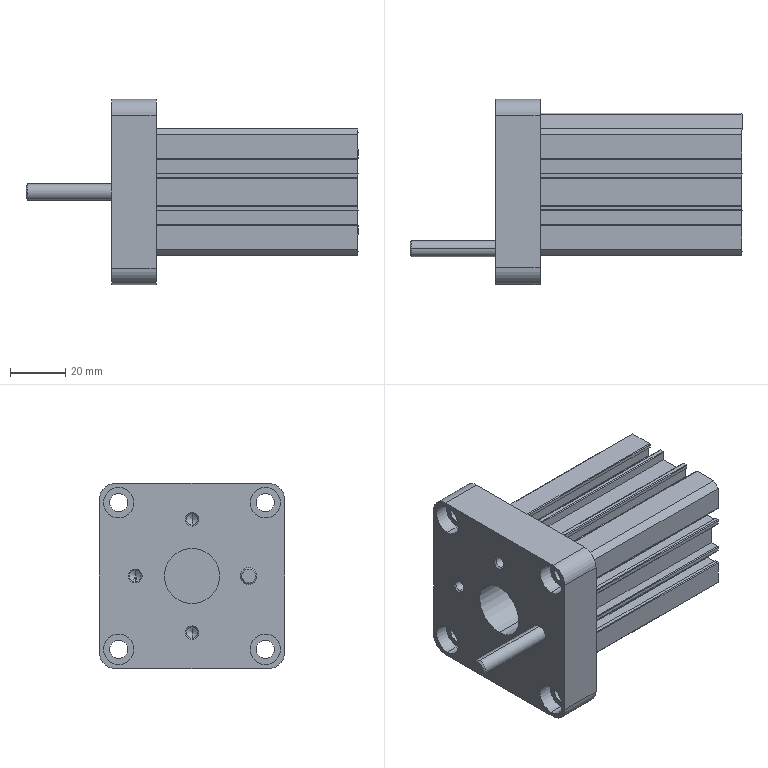Part | STEP file | 1105WWT1_2 | 1 solid | 207 faces | box 120 x 67 x 67 mm | volume 176582 mm3 | plane 105 | cylinder 78 | cone 24 | commonest cylinder face diameters 0.6 x18 11 x16 4.134 x8 6.6 x8 8.566 x4 10 x4